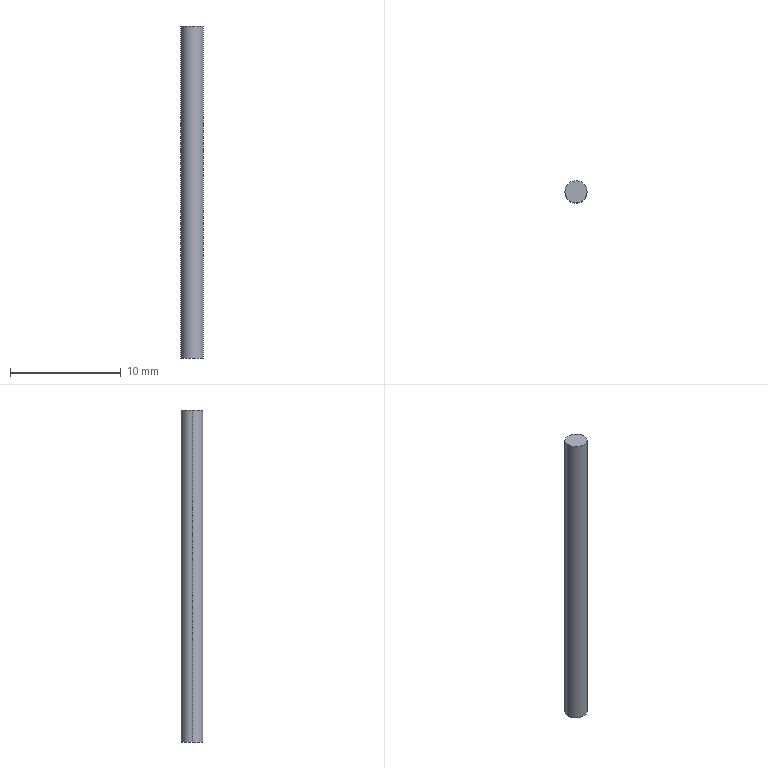Part | SolidWorks | features Extrusion 1 | 1 solid | 4 faces | box 2 x 2 x 30 mm | volume 94.248 mm3 | cylinder 2 | plane 2 | commonest cylinder face diameters 2 x2
STEP:
#1=CARTESIAN_POINT('',(1.,0.,30.));
#2=VERTEX_POINT('',#1);
#3=CARTESIAN_POINT('',(-1.,0.,30.));
#4=VERTEX_POINT('',#3);
#5=CARTESIAN_POINT('',(0.,0.,30.));
#6=DIRECTION('',(0.,0.,1.));
#7=DIRECTION('',(1.,0.,0.));
#8=AXIS2_PLACEMENT_3D('',#5,#6,#7);
#9=CIRCLE('',#8,1.);
#10=EDGE_CURVE('',#2,#4,#9,.T.);
#11=ORIENTED_EDGE('',*,*,#10,.F.);
#12=CARTESIAN_POINT('',(1.,0.,0.));
#13=VERTEX_POINT('',#12);
#14=CARTESIAN_POINT('',(1.,0.,30.));
#15=DIRECTION('',(0.,0.,-1.));
#16=VECTOR('',#15,1000.);
#17=LINE('',#14,#16);
#18=EDGE_CURVE('',#2,#13,#17,.T.);
#19=ORIENTED_EDGE('',*,*,#18,.T.);
#20=CARTESIAN_POINT('',(-1.,0.,0.));
#21=VERTEX_POINT('',#20);
#22=CARTESIAN_POINT('',(0.,0.,0.));
#23=DIRECTION('',(0.,0.,1.));
#24=DIRECTION('',(1.,0.,0.));
#25=AXIS2_PLACEMENT_3D('',#22,#23,#24);
#26=CIRCLE('',#25,1.);
#27=EDGE_CURVE('',#13,#21,#26,.T.);
#28=ORIENTED_EDGE('',*,*,#27,.T.);
#29=CARTESIAN_POINT('',(-1.,0.,30.));
#30=DIRECTION('',(0.,0.,-1.));
#31=VECTOR('',#30,1000.);
#32=LINE('',#29,#31);
#33=EDGE_CURVE('',#4,#21,#32,.T.);
#34=ORIENTED_EDGE('',*,*,#33,.F.);
#35=EDGE_LOOP('',(#11,#19,#28,#34));
#36=FACE_OUTER_BOUND('',#35,.T.);
#37=CARTESIAN_POINT('',(0.,0.,30.));
#38=DIRECTION('',(0.,0.,-1.));
#39=DIRECTION('',(-1.,0.,0.));
#40=AXIS2_PLACEMENT_3D('',#37,#38,#39);
#41=CYLINDRICAL_SURFACE('',#40,1.);
#42=ADVANCED_FACE('',(#36),#41,.T.);
#43=ORIENTED_EDGE('',*,*,#18,.F.);
#44=CARTESIAN_POINT('',(0.,0.,30.));
#45=DIRECTION('',(0.,0.,1.));
#46=DIRECTION('',(1.,0.,0.));
#47=AXIS2_PLACEMENT_3D('',#44,#45,#46);
#48=CIRCLE('',#47,1.);
#49=EDGE_CURVE('',#4,#2,#48,.T.);
#50=ORIENTED_EDGE('',*,*,#49,.F.);
#51=ORIENTED_EDGE('',*,*,#33,.T.);
#52=CARTESIAN_POINT('',(0.,0.,0.));
#53=DIRECTION('',(0.,0.,1.));
#54=DIRECTION('',(1.,0.,0.));
#55=AXIS2_PLACEMENT_3D('',#52,#53,#54);
#56=CIRCLE('',#55,1.);
#57=EDGE_CURVE('',#21,#13,#56,.T.);
#58=ORIENTED_EDGE('',*,*,#57,.T.);
#59=EDGE_LOOP('',(#43,#50,#51,#58));
#60=FACE_OUTER_BOUND('',#59,.T.);
#61=CARTESIAN_POINT('',(0.,0.,30.));
#62=DIRECTION('',(0.,0.,-1.));
#63=DIRECTION('',(-1.,0.,0.));
#64=AXIS2_PLACEMENT_3D('',#61,#62,#63);
#65=CYLINDRICAL_SURFACE('',#64,1.);
#66=ADVANCED_FACE('',(#60),#65,.T.);
#67=ORIENTED_EDGE('',*,*,#49,.T.);
#68=ORIENTED_EDGE('',*,*,#10,.T.);
#69=EDGE_LOOP('',(#67,#68));
#70=FACE_OUTER_BOUND('',#69,.T.);
#71=CARTESIAN_POINT('',(0.,0.,30.));
#72=DIRECTION('',(0.,0.,1.));
#73=DIRECTION('',(1.,0.,0.));
#74=AXIS2_PLACEMENT_3D('',#71,#72,#73);
#75=PLANE('',#74);
#76=ADVANCED_FACE('',(#70),#75,.T.);
#77=ORIENTED_EDGE('',*,*,#57,.F.);
#78=ORIENTED_EDGE('',*,*,#27,.F.);
#79=EDGE_LOOP('',(#77,#78));
#80=FACE_OUTER_BOUND('',#79,.T.);
#81=CARTESIAN_POINT('',(0.,0.,0.));
#82=DIRECTION('',(0.,0.,1.));
#83=DIRECTION('',(1.,0.,0.));
#84=AXIS2_PLACEMENT_3D('',#81,#82,#83);
#85=PLANE('',#84);
#86=ADVANCED_FACE('',(#80),#85,.F.);
#87=CLOSED_SHELL('',(#42,#66,#76,#86));
#88=MANIFOLD_SOLID_BREP('',#87);
#89=CARTESIAN_POINT('',(0.,0.,0.));
#90=DIRECTION('',(0.,0.,1.));
#91=DIRECTION('',(1.,0.,0.));
#92=AXIS2_PLACEMENT_3D('',#89,#90,#91);
#93=(LENGTH_UNIT()NAMED_UNIT(*)SI_UNIT(.MILLI.,.METRE.));
#94=UNCERTAINTY_MEASURE_WITH_UNIT(LENGTH_MEASURE(0.00001),#93,'','');
#95=(NAMED_UNIT(*)PLANE_ANGLE_UNIT()SI_UNIT($,.RADIAN.));
#96=(NAMED_UNIT(*)SI_UNIT($,.STERADIAN.)SOLID_ANGLE_UNIT());
#97=(GEOMETRIC_REPRESENTATION_CONTEXT(3)GLOBAL_UNCERTAINTY_ASSIGNED_CONTEXT((#94))GLOBAL_UNIT_ASSIGNED_CONTEXT((#93,#95,#96))REPRESENTATION_CONTEXT('',''));
#98=ADVANCED_BREP_SHAPE_REPRESENTATION('',(#88,#92),#97);